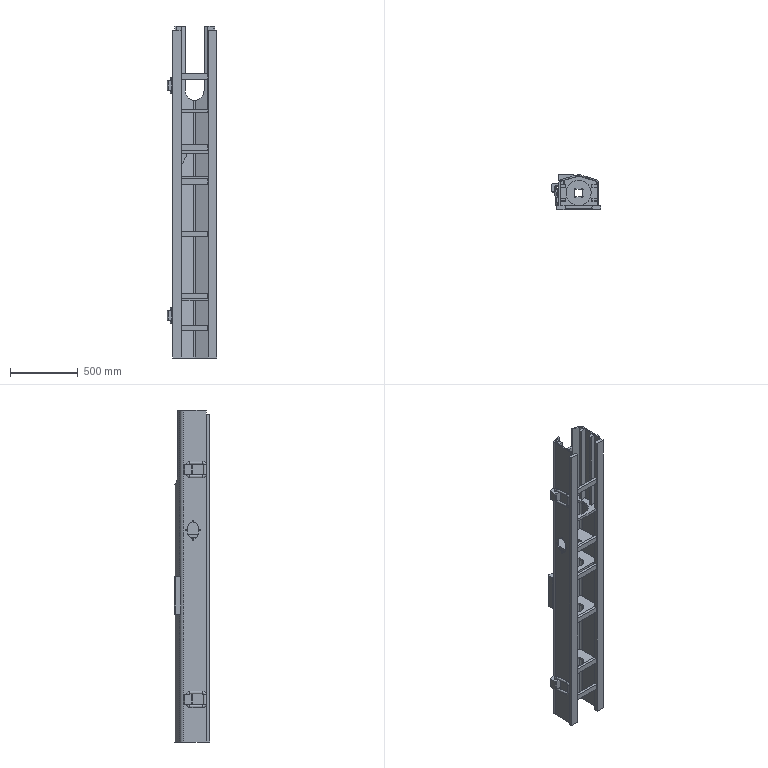Part | SolidWorks | features LocalLPattern 11, ReferencePattern 11, MateUpdatePoint 2 | 25 solids | 302 faces | box 364.5 x 260.017 x 2455 mm | volume 31232194 mm3 | plane 197 | cylinder 81 | torus 16 | cone 8 | commonest cylinder face diameters 20 x20 50 x10 8.5 x8 10.2 x8 70 x8 12 x6